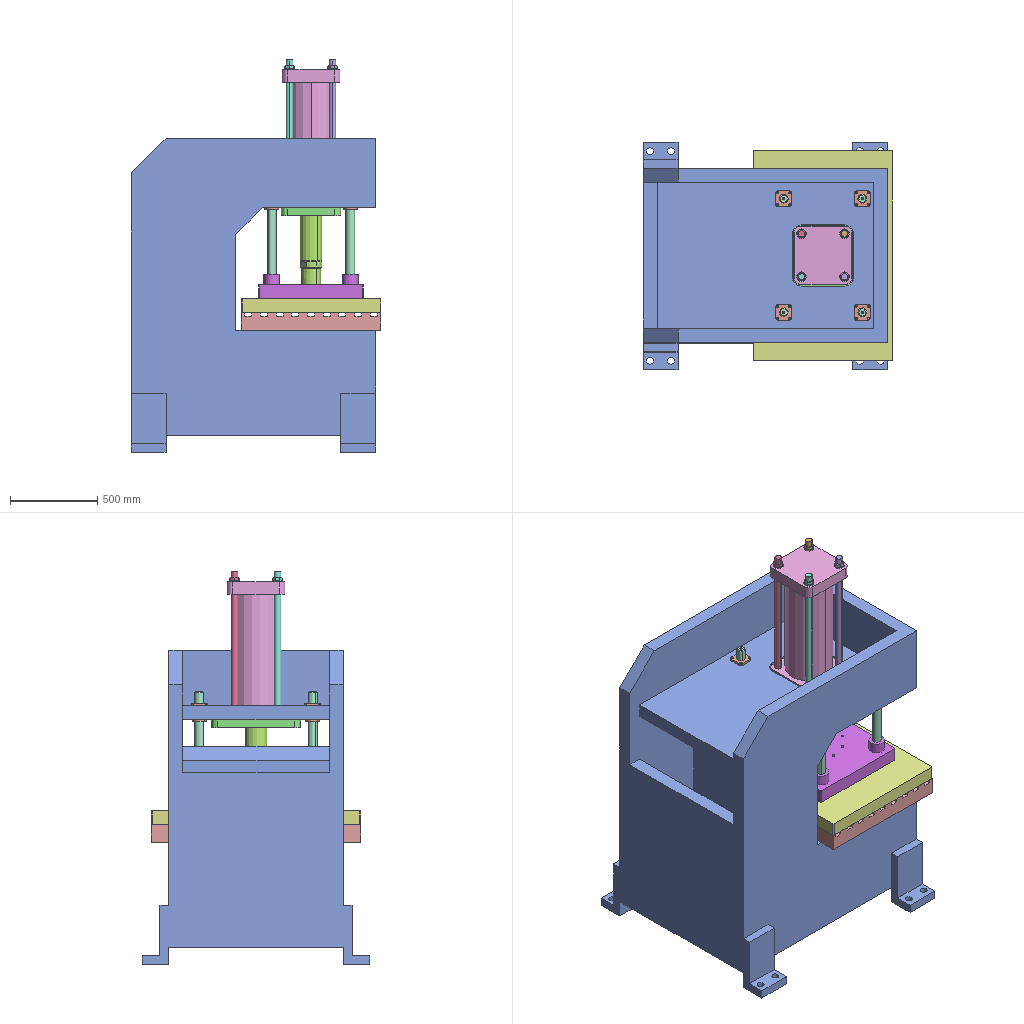Assembly | SolidWorks | 8 different items | 14 placed | box 1430 x 1300 x 2249 mm
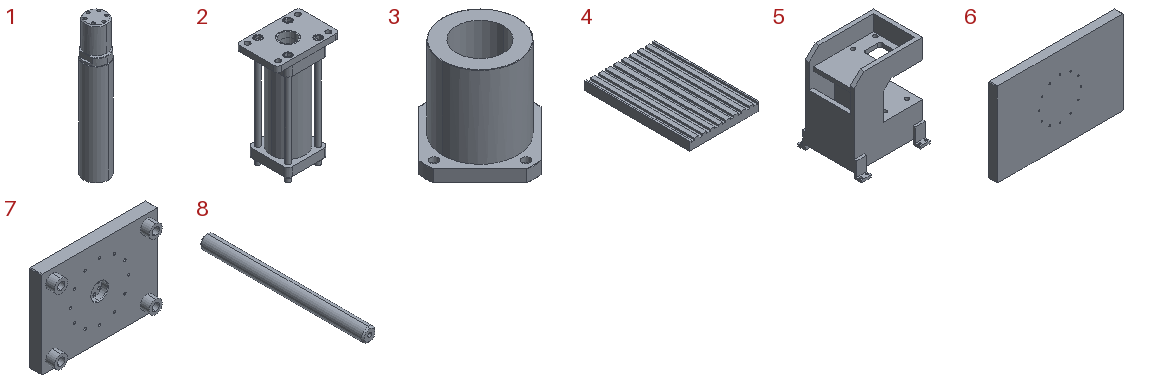Parts list (item | quantity | size | volume | features):
1 | x1 | 125 x 125 x 690 mm | 7968385 mm3 | features BaseBody 1, CirPattern 1, HoleWzd 1
2 | x1 | 510 x 340 x 894.436 mm | 57179698 mm3 | features BaseBody 7
3 | x4 | 116 x 116 x 100 mm | 342037 mm3 | features BaseBody 1
4 | x1 | 800 x 1200 x 100 mm | 87360000 mm3 | features Extrusion 1, ICE 1, LPattern 1
5 | x1 | 1400 x 1300 x 1800 mm | 599795931 mm3 | features ICE 6, Chamfer 2, Cut 2, MirrorPattern 2, Extrusion 1, Fillet 1, MoveFace 1, Shell 1
6 | x1 | 1200 x 80 x 800 mm | 76723214 mm3 | features Chamfer 1, Extrusion 1, HoleWzd 1
7 | x1 | 800 x 140 x 600 mm | 38677043 mm3 | features ICE 3, Chamfer 2, HoleWzd 2, CirPattern 1, Extrusion 1
8 | x4 | 50 x 600 x 50 mm | 1162301 mm3 | features HoleWzd 2, Chamfer 1, Extrusion 1
Mates (type | each side: item.copy, entity, surface, feature):
Width | 4.1 face plane Boss-Extrude1 | 4.1 face plane Boss-Extrude1 | 5.1 face plane Boss-Extrude1 | 5.1 face plane Boss-Extrude1
Coincident | 4.1 face plane Boss-Extrude1 | 5.1 face plane Cut-Extrude1
DistanceDim | 4.1 face plane Boss-Extrude1 | 5.1 face plane Boss-Extrude1
Width | 5.1 face plane Boss-Extrude1 | 5.1 face plane Boss-Extrude1 | 2.1 face plane Input5 | 2.1 face plane Input5
Coincident | 5.1 face plane Cut-Extrude1 | 2.1 face plane Input5
Concentric | 1.1 face cylinder Input1 | 2.1 face cylinder Input7
Width | 4.1 face plane Boss-Extrude1 | 4.1 face plane Boss-Extrude1 | 2.1 face cylinder Input1
Width | 4.1 face plane Boss-Extrude1 | 4.1 face plane Boss-Extrude1 | 6.1 face plane Boss-Extrude1 | 6.1 face plane Boss-Extrude1 | 2 times
Width | 6.1 face plane Boss-Extrude1 | 6.1 face plane Boss-Extrude1 | 7.1 face plane Boss-Extrude1 | 7.1 face plane Boss-Extrude1 | 2 times
Coincident | 6.1 face plane Boss-Extrude1 | 7.1 face plane Boss-Extrude1
Coincident | 1.1 face plane Input1 | 7.1 face plane Cut-Extrude1
Concentric | 7.1 face cylinder Boss-Extrude2 | 8.1 face cylinder Boss-Extrude1
Coincident | 7.1 face plane Boss-Extrude1 | 8.1 face plane Boss-Extrude1
Concentric | 7.1 face cylinder Boss-Extrude2 | 8.2 face cylinder Boss-Extrude1
Coincident | 8.1 face plane Boss-Extrude1 | 8.2 face plane Boss-Extrude1
Concentric | 7.1 face cylinder Boss-Extrude2 | 8.3 face cylinder Boss-Extrude1
Coincident | 8.2 face plane Boss-Extrude1 | 8.3 face plane Boss-Extrude1
Coincident | 8.4 face plane Boss-Extrude1 | 8.2 face plane Boss-Extrude1
Concentric | 7.1 face cylinder Boss-Extrude2 | 8.4 face cylinder Boss-Extrude1
Concentric | 8.3 face cylinder Boss-Extrude1 | 3.1 face cylinder Input1
Coincident | 5.1 face plane Shell1 | 3.1 face plane Input1
Concentric | 8.4 face cylinder Boss-Extrude1 | 3.2 face cylinder Input1
Coincident | 5.1 face plane Shell1 | 3.2 face plane Input1
Concentric | 8.1 face cylinder Boss-Extrude1 | 3.3 face cylinder Input1
Coincident | 3.2 face plane Input1 | 3.3 face plane Input1 | 2 times
Concentric | 8.2 face cylinder Boss-Extrude1 | 3.4 face cylinder Input1
Coincident | 3.1 face plane Input1 | 3.4 face plane Input1 | 2 times
Parallel | 3.1 face plane Input1 | 3.2 face plane Input1
LimitDistanceDim | 6.1 face plane Boss-Extrude1 | 4.1 face plane Boss-Extrude1